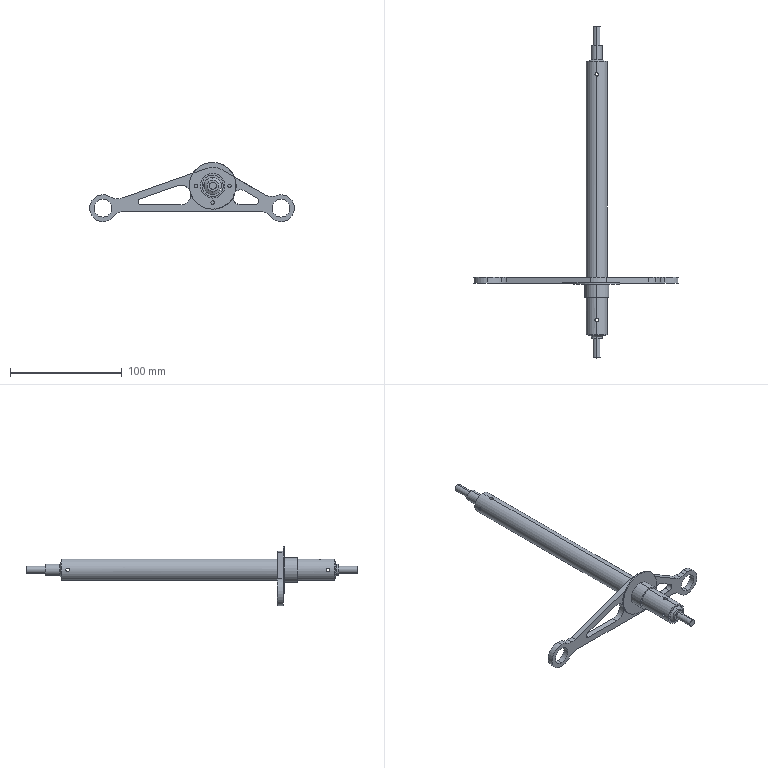Part | SolidWorks | features BaseBody 3 | 3 solids | 119 faces | box 183 x 296.652 x 52.955 mm | volume 44712 mm3 | cylinder 85 | plane 26 | cone 8 | commonest cylinder face diameters 3.2 x38 24 x6 25.4 x6 6.35 x4 10.16 x4 15.24 x4